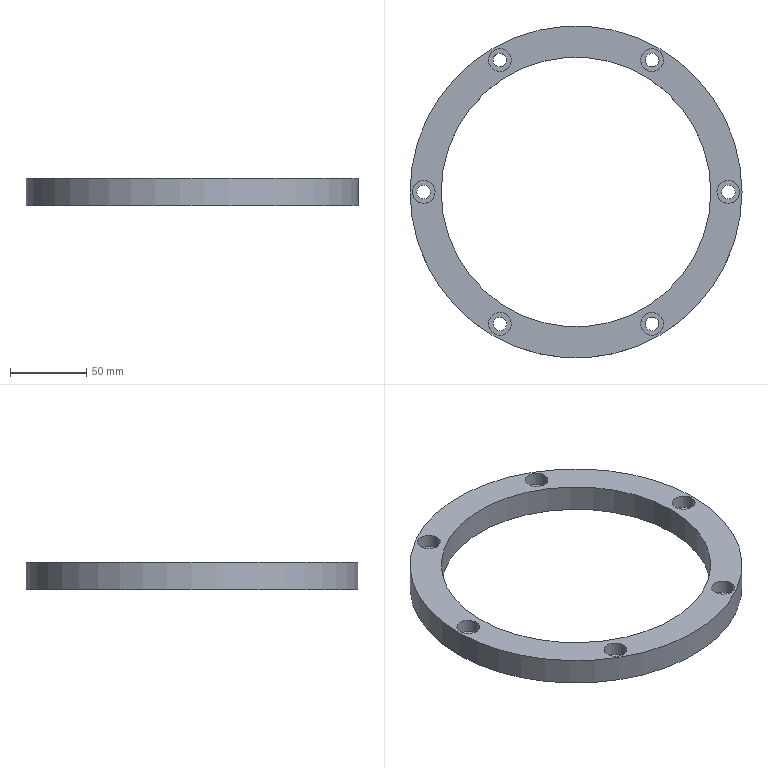CAM job | NX | 3-axis milling, drilling | part box 218 x 218 x 18 mm | stock box 218 x 218 x 18 mm
Tools:
number,name,description,diameter,corner_radius,flute_length,length,flutes
7,D6A45,Milling Tool-5 Parameters,6.0,0.0,3.0,3.0,2
1,ZXZ,Milling Tool-5 Parameters,6.0,0.0,50.0,75.0,2
9,9.0ZT,Drilling Tool,9.0,0.0,35.0,50.0,2
10,D10,Milling Tool-5 Parameters,10.0,0.0,50.0,75.0,2
Operations:
program,operation,operation_type,tool,method,geometry_group,spindle_rpm,surface_speed,feed_per_tooth,feed_cut,feed_plunge,cut_length_mm,path_length_mm,cut_time_min,machine_time_min
1,DRILLING,Operation,ZXZ,METHOD,A,3000.0,56.0,0.0333,200.0,0.0,24.0,623.225,0.12,0.1799
1,DRILLING_COPY,Operation,9.0ZT,METHOD,A,1203.0,34.0,0.0623,150.0,0.0,151.223,877.671,1.008,1.081
1,HOLE_MILLING,CylinderMilling,D10,METHOD,A,3000.0,94.0,0.3333,2000.0,100.0,4618.504,5529.504,2.309,2.4
1,ZLEVEL_PROFILE_1_COPY_1,ZLevelMilling,D6A45,METHOD,A,6500.0,122.0,0.0769,1000.0,100.0,283.315,1268.482,0.2833,0.3818